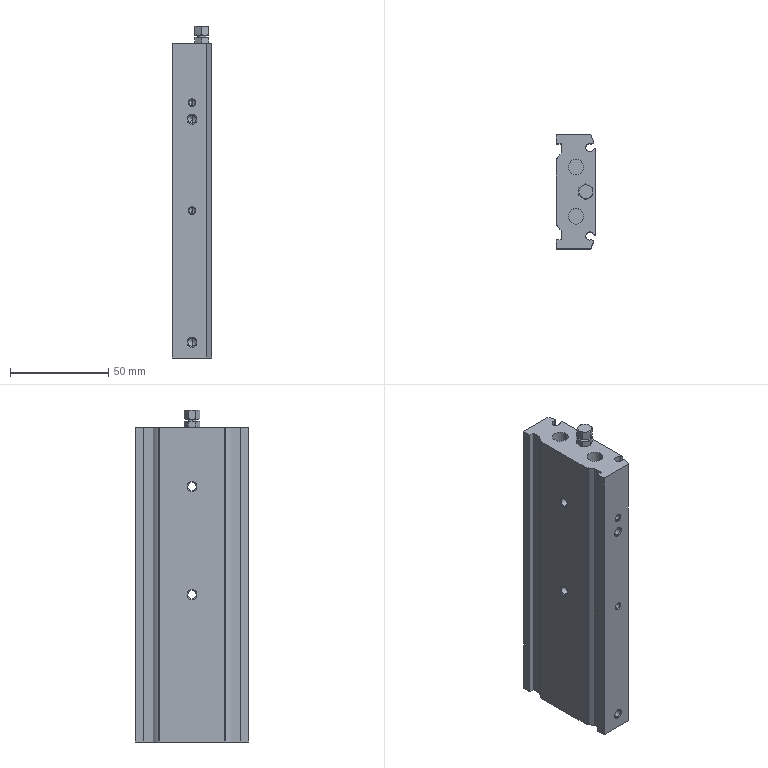Part | SolidWorks | features BaseBody 1 | 1 solid | 139 faces | box 20 x 58 x 169 mm | volume 126513 mm3 | cone 60 | plane 41 | cylinder 38 | commonest cylinder face diameters 3.242 x8 4.134 x8 8 x8 4.3 x4 16 x4 4 x2